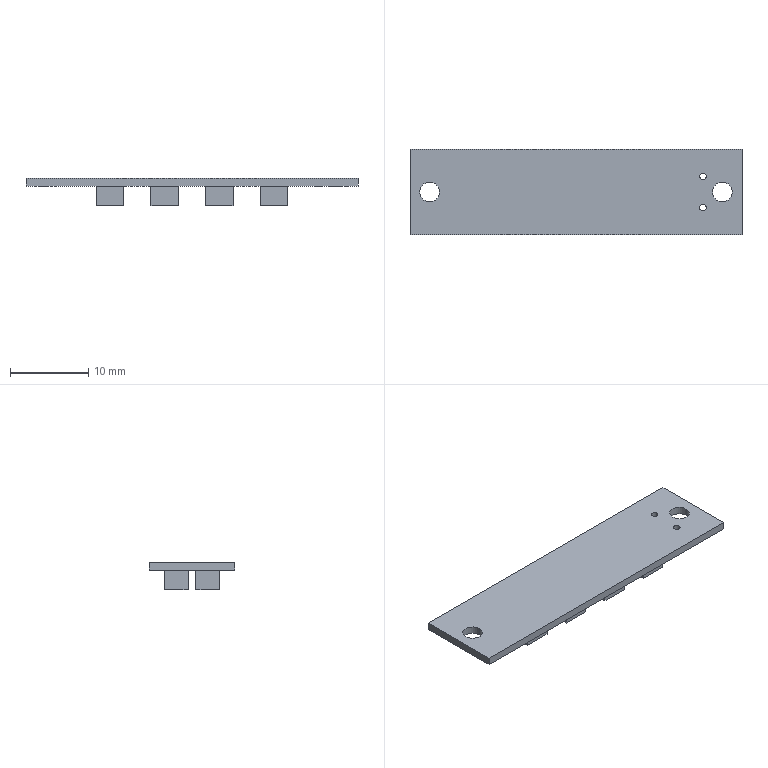Part | STEP file | LED lamp | 1 solid | 54 faces | box 42.5 x 11 x 3.5 mm | volume 662.951 mm3 | plane 46 | cylinder 8 | commonest cylinder face diameters 2.5 x4 0.838 x2 0.855 x2
STEP:
#1=CARTESIAN_POINT('',(27.178,-4.,3.5));
#2=VERTEX_POINT('',#1);
#3=CARTESIAN_POINT('',(26.322,-4.,3.5));
#4=VERTEX_POINT('',#3);
#5=CARTESIAN_POINT('',(26.75,-4.,3.5));
#6=DIRECTION('',(0.,0.,-1.));
#7=DIRECTION('',(-1.,0.,0.));
#8=AXIS2_PLACEMENT_3D('',#5,#6,#7);
#9=CIRCLE('',#8,0.4275);
#10=EDGE_CURVE('',#2,#4,#9,.T.);
#11=ORIENTED_EDGE('',*,*,#10,.F.);
#12=CARTESIAN_POINT('',(27.178,-4.,2.5));
#13=VERTEX_POINT('',#12);
#14=CARTESIAN_POINT('',(27.178,-4.,3.5));
#15=DIRECTION('',(0.,0.,-1.));
#16=VECTOR('',#15,1000.);
#17=LINE('',#14,#16);
#18=EDGE_CURVE('',#2,#13,#17,.T.);
#19=ORIENTED_EDGE('',*,*,#18,.T.);
#20=CARTESIAN_POINT('',(26.322,-4.,2.5));
#21=VERTEX_POINT('',#20);
#22=CARTESIAN_POINT('',(26.75,-4.,2.5));
#23=DIRECTION('',(0.,0.,-1.));
#24=DIRECTION('',(-1.,0.,0.));
#25=AXIS2_PLACEMENT_3D('',#22,#23,#24);
#26=CIRCLE('',#25,0.4275);
#27=EDGE_CURVE('',#13,#21,#26,.T.);
#28=ORIENTED_EDGE('',*,*,#27,.T.);
#29=CARTESIAN_POINT('',(26.322,-4.,3.5));
#30=DIRECTION('',(0.,0.,-1.));
#31=VECTOR('',#30,1000.);
#32=LINE('',#29,#31);
#33=EDGE_CURVE('',#4,#21,#32,.T.);
#34=ORIENTED_EDGE('',*,*,#33,.F.);
#35=EDGE_LOOP('',(#11,#19,#28,#34));
#36=FACE_OUTER_BOUND('',#35,.T.);
#37=CARTESIAN_POINT('',(26.75,-4.,3.5));
#38=DIRECTION('',(0.,0.,-1.));
#39=DIRECTION('',(-1.,0.,0.));
#40=AXIS2_PLACEMENT_3D('',#37,#38,#39);
#41=CYLINDRICAL_SURFACE('',#40,0.4275);
#42=ADVANCED_FACE('',(#36),#41,.F.);
#43=CARTESIAN_POINT('',(27.169,0.,3.5));
#44=VERTEX_POINT('',#43);
#45=CARTESIAN_POINT('',(26.331,0.,3.5));
#46=VERTEX_POINT('',#45);
#47=CARTESIAN_POINT('',(26.75,0.,3.5));
#48=DIRECTION('',(0.,0.,-1.));
#49=DIRECTION('',(-1.,0.,0.));
#50=AXIS2_PLACEMENT_3D('',#47,#48,#49);
#51=CIRCLE('',#50,0.4192);
#52=EDGE_CURVE('',#44,#46,#51,.T.);
#53=ORIENTED_EDGE('',*,*,#52,.F.);
#54=CARTESIAN_POINT('',(27.169,0.,2.5));
#55=VERTEX_POINT('',#54);
#56=CARTESIAN_POINT('',(27.169,0.,3.5));
#57=DIRECTION('',(0.,0.,-1.));
#58=VECTOR('',#57,1000.);
#59=LINE('',#56,#58);
#60=EDGE_CURVE('',#44,#55,#59,.T.);
#61=ORIENTED_EDGE('',*,*,#60,.T.);
#62=CARTESIAN_POINT('',(26.331,0.,2.5));
#63=VERTEX_POINT('',#62);
#64=CARTESIAN_POINT('',(26.75,0.,2.5));
#65=DIRECTION('',(0.,0.,-1.));
#66=DIRECTION('',(-1.,0.,0.));
#67=AXIS2_PLACEMENT_3D('',#64,#65,#66);
#68=CIRCLE('',#67,0.4192);
#69=EDGE_CURVE('',#55,#63,#68,.T.);
#70=ORIENTED_EDGE('',*,*,#69,.T.);
#71=CARTESIAN_POINT('',(26.331,0.,3.5));
#72=DIRECTION('',(0.,0.,-1.));
#73=VECTOR('',#72,1000.);
#74=LINE('',#71,#73);
#75=EDGE_CURVE('',#46,#63,#74,.T.);
#76=ORIENTED_EDGE('',*,*,#75,.F.);
#77=EDGE_LOOP('',(#53,#61,#70,#76));
#78=FACE_OUTER_BOUND('',#77,.T.);
#79=CARTESIAN_POINT('',(26.75,0.,3.5));
#80=DIRECTION('',(0.,0.,-1.));
#81=DIRECTION('',(-1.,0.,0.));
#82=AXIS2_PLACEMENT_3D('',#79,#80,#81);
#83=CYLINDRICAL_SURFACE('',#82,0.4192);
#84=ADVANCED_FACE('',(#78),#83,.F.);
#85=CARTESIAN_POINT('',(-7.,-2.,3.5));
#86=VERTEX_POINT('',#85);
#87=CARTESIAN_POINT('',(-9.5,-2.,3.5));
#88=VERTEX_POINT('',#87);
#89=CARTESIAN_POINT('',(-8.25,-2.,3.5));
#90=DIRECTION('',(0.,0.,-1.));
#91=DIRECTION('',(-1.,0.,0.));
#92=AXIS2_PLACEMENT_3D('',#89,#90,#91);
#93=CIRCLE('',#92,1.25);
#94=EDGE_CURVE('',#86,#88,#93,.T.);
#95=ORIENTED_EDGE('',*,*,#94,.F.);
#96=CARTESIAN_POINT('',(-7.,-2.,2.5));
#97=VERTEX_POINT('',#96);
#98=CARTESIAN_POINT('',(-7.,-2.,3.5));
#99=DIRECTION('',(0.,0.,-1.));
#100=VECTOR('',#99,1000.);
#101=LINE('',#98,#100);
#102=EDGE_CURVE('',#86,#97,#101,.T.);
#103=ORIENTED_EDGE('',*,*,#102,.T.);
#104=CARTESIAN_POINT('',(-9.5,-2.,2.5));
#105=VERTEX_POINT('',#104);
#106=CARTESIAN_POINT('',(-8.25,-2.,2.5));
#107=DIRECTION('',(0.,0.,-1.));
#108=DIRECTION('',(-1.,0.,0.));
#109=AXIS2_PLACEMENT_3D('',#106,#107,#108);
#110=CIRCLE('',#109,1.25);
#111=EDGE_CURVE('',#97,#105,#110,.T.);
#112=ORIENTED_EDGE('',*,*,#111,.T.);
#113=CARTESIAN_POINT('',(-9.5,-2.,3.5));
#114=DIRECTION('',(0.,0.,-1.));
#115=VECTOR('',#114,1000.);
#116=LINE('',#113,#115);
#117=EDGE_CURVE('',#88,#105,#116,.T.);
#118=ORIENTED_EDGE('',*,*,#117,.F.);
#119=EDGE_LOOP('',(#95,#103,#112,#118));
#120=FACE_OUTER_BOUND('',#119,.T.);
#121=CARTESIAN_POINT('',(-8.25,-2.,3.5));
#122=DIRECTION('',(0.,0.,-1.));
#123=DIRECTION('',(-1.,0.,0.));
#124=AXIS2_PLACEMENT_3D('',#121,#122,#123);
#125=CYLINDRICAL_SURFACE('',#124,1.25);
#126=ADVANCED_FACE('',(#120),#125,.F.);
#127=CARTESIAN_POINT('',(30.5,-2.,3.5));
#128=VERTEX_POINT('',#127);
#129=CARTESIAN_POINT('',(28.,-2.,3.5));
#130=VERTEX_POINT('',#129);
#131=CARTESIAN_POINT('',(29.25,-2.,3.5));
#132=DIRECTION('',(0.,0.,-1.));
#133=DIRECTION('',(-1.,0.,0.));
#134=AXIS2_PLACEMENT_3D('',#131,#132,#133);
#135=CIRCLE('',#134,1.25);
#136=EDGE_CURVE('',#128,#130,#135,.T.);
#137=ORIENTED_EDGE('',*,*,#136,.F.);
#138=CARTESIAN_POINT('',(30.5,-2.,2.5));
#139=VERTEX_POINT('',#138);
#140=CARTESIAN_POINT('',(30.5,-2.,3.5));
#141=DIRECTION('',(0.,0.,-1.));
#142=VECTOR('',#141,1000.);
#143=LINE('',#140,#142);
#144=EDGE_CURVE('',#128,#139,#143,.T.);
#145=ORIENTED_EDGE('',*,*,#144,.T.);
#146=CARTESIAN_POINT('',(28.,-2.,2.5));
#147=VERTEX_POINT('',#146);
#148=CARTESIAN_POINT('',(29.25,-2.,2.5));
#149=DIRECTION('',(0.,0.,-1.));
#150=DIRECTION('',(-1.,0.,0.));
#151=AXIS2_PLACEMENT_3D('',#148,#149,#150);
#152=CIRCLE('',#151,1.25);
#153=EDGE_CURVE('',#139,#147,#152,.T.);
#154=ORIENTED_EDGE('',*,*,#153,.T.);
#155=CARTESIAN_POINT('',(28.,-2.,3.5));
#156=DIRECTION('',(0.,0.,-1.));
#157=VECTOR('',#156,1000.);
#158=LINE('',#155,#157);
#159=EDGE_CURVE('',#130,#147,#158,.T.);
#160=ORIENTED_EDGE('',*,*,#159,.F.);
#161=EDGE_LOOP('',(#137,#145,#154,#160));
#162=FACE_OUTER_BOUND('',#161,.T.);
#163=CARTESIAN_POINT('',(29.25,-2.,3.5));
#164=DIRECTION('',(0.,0.,-1.));
#165=DIRECTION('',(-1.,0.,0.));
#166=AXIS2_PLACEMENT_3D('',#163,#164,#165);
#167=CYLINDRICAL_SURFACE('',#166,1.25);
#168=ADVANCED_FACE('',(#162),#167,.F.);
#169=CARTESIAN_POINT('',(26.75,-4.,2.5));
#170=DIRECTION('',(0.,0.,-1.));
#171=DIRECTION('',(-1.,0.,0.));
#172=AXIS2_PLACEMENT_3D('',#169,#170,#171);
#173=CIRCLE('',#172,0.4275);
#174=EDGE_CURVE('',#21,#13,#173,.T.);
#175=ORIENTED_EDGE('',*,*,#174,.F.);
#176=ORIENTED_EDGE('',*,*,#27,.F.);
#177=EDGE_LOOP('',(#175,#176));
#178=FACE_BOUND('',#177,.T.);
#179=CARTESIAN_POINT('',(26.75,0.,2.5));
#180=DIRECTION('',(0.,0.,-1.));
#181=DIRECTION('',(-1.,0.,0.));
#182=AXIS2_PLACEMENT_3D('',#179,#180,#181);
#183=CIRCLE('',#182,0.4192);
#184=EDGE_CURVE('',#63,#55,#183,.T.);
#185=ORIENTED_EDGE('',*,*,#184,.F.);
#186=ORIENTED_EDGE('',*,*,#69,.F.);
#187=EDGE_LOOP('',(#185,#186));
#188=FACE_BOUND('',#187,.T.);
#189=CARTESIAN_POINT('',(-8.25,-2.,2.5));
#190=DIRECTION('',(0.,0.,-1.));
#191=DIRECTION('',(-1.,0.,0.));
#192=AXIS2_PLACEMENT_3D('',#189,#190,#191);
#193=CIRCLE('',#192,1.25);
#194=EDGE_CURVE('',#105,#97,#193,.T.);
#195=ORIENTED_EDGE('',*,*,#194,.F.);
#196=ORIENTED_EDGE('',*,*,#111,.F.);
#197=EDGE_LOOP('',(#195,#196));
#198=FACE_BOUND('',#197,.T.);
#199=CARTESIAN_POINT('',(29.25,-2.,2.5));
#200=DIRECTION('',(0.,0.,-1.));
#201=DIRECTION('',(-1.,0.,0.));
#202=AXIS2_PLACEMENT_3D('',#199,#200,#201);
#203=CIRCLE('',#202,1.25);
#204=EDGE_CURVE('',#147,#139,#203,.T.);
#205=ORIENTED_EDGE('',*,*,#204,.F.);
#206=ORIENTED_EDGE('',*,*,#153,.F.);
#207=EDGE_LOOP('',(#205,#206));
#208=FACE_BOUND('',#207,.T.);
#209=CARTESIAN_POINT('',(12.25,-2.637,2.5));
#210=VERTEX_POINT('',#209);
#211=CARTESIAN_POINT('',(12.25,-5.5,2.5));
#212=VERTEX_POINT('',#211);
#213=CARTESIAN_POINT('',(12.25,-2.637,2.5));
#214=DIRECTION('',(0.,-1.,0.));
#215=VECTOR('',#214,1000.);
#216=LINE('',#213,#215);
#217=EDGE_CURVE('',#210,#212,#216,.T.);
#218=ORIENTED_EDGE('',*,*,#217,.T.);
#219=CARTESIAN_POINT('',(15.75,-5.5,2.5));
#220=VERTEX_POINT('',#219);
#221=CARTESIAN_POINT('',(12.25,-5.5,2.5));
#222=DIRECTION('',(1.,0.,0.));
#223=VECTOR('',#222,1000.);
#224=LINE('',#221,#223);
#225=EDGE_CURVE('',#212,#220,#224,.T.);
#226=ORIENTED_EDGE('',*,*,#225,.T.);
#227=CARTESIAN_POINT('',(15.75,-2.637,2.5));
#228=VERTEX_POINT('',#227);
#229=CARTESIAN_POINT('',(15.75,-2.637,2.5));
#230=DIRECTION('',(0.,1.,0.));
#231=VECTOR('',#230,1000.);
#232=LINE('',#229,#231);
#233=EDGE_CURVE('',#220,#228,#232,.T.);
#234=ORIENTED_EDGE('',*,*,#233,.T.);
#235=CARTESIAN_POINT('',(12.25,-2.637,2.5));
#236=DIRECTION('',(-1.,0.,0.));
#237=VECTOR('',#236,1000.);
#238=LINE('',#235,#237);
#239=EDGE_CURVE('',#228,#210,#238,.T.);
#240=ORIENTED_EDGE('',*,*,#239,.T.);
#241=EDGE_LOOP('',(#218,#226,#234,#240));
#242=FACE_BOUND('',#241,.T.);
#243=CARTESIAN_POINT('',(-1.75,-2.5,2.5));
#244=VERTEX_POINT('',#243);
#245=CARTESIAN_POINT('',(-1.75,-5.5,2.5));
#246=VERTEX_POINT('',#245);
#247=CARTESIAN_POINT('',(-1.75,-2.5,2.5));
#248=DIRECTION('',(0.,-1.,0.));
#249=VECTOR('',#248,1000.);
#250=LINE('',#247,#249);
#251=EDGE_CURVE('',#244,#246,#250,.T.);
#252=ORIENTED_EDGE('',*,*,#251,.T.);
#253=CARTESIAN_POINT('',(1.75,-5.5,2.5));
#254=VERTEX_POINT('',#253);
#255=CARTESIAN_POINT('',(-1.75,-5.5,2.5));
#256=DIRECTION('',(1.,0.,0.));
#257=VECTOR('',#256,1000.);
#258=LINE('',#255,#257);
#259=EDGE_CURVE('',#246,#254,#258,.T.);
#260=ORIENTED_EDGE('',*,*,#259,.T.);
#261=CARTESIAN_POINT('',(1.75,-2.5,2.5));
#262=VERTEX_POINT('',#261);
#263=CARTESIAN_POINT('',(1.75,-2.5,2.5));
#264=DIRECTION('',(0.,1.,0.));
#265=VECTOR('',#264,1000.);
#266=LINE('',#263,#265);
#267=EDGE_CURVE('',#254,#262,#266,.T.);
#268=ORIENTED_EDGE('',*,*,#267,.T.);
#269=CARTESIAN_POINT('',(-1.75,-2.5,2.5));
#270=DIRECTION('',(-1.,0.,0.));
#271=VECTOR('',#270,1000.);
#272=LINE('',#269,#271);
#273=EDGE_CURVE('',#262,#244,#272,.T.);
#274=ORIENTED_EDGE('',*,*,#273,.T.);
#275=EDGE_LOOP('',(#252,#260,#268,#274));
#276=FACE_BOUND('',#275,.T.);
#277=CARTESIAN_POINT('',(12.25,1.5,2.5));
#278=VERTEX_POINT('',#277);
#279=CARTESIAN_POINT('',(12.25,-1.5,2.5));
#280=VERTEX_POINT('',#279);
#281=CARTESIAN_POINT('',(12.25,1.5,2.5));
#282=DIRECTION('',(0.,-1.,0.));
#283=VECTOR('',#282,1000.);
#284=LINE('',#281,#283);
#285=EDGE_CURVE('',#278,#280,#284,.T.);
#286=ORIENTED_EDGE('',*,*,#285,.T.);
#287=CARTESIAN_POINT('',(15.75,-1.5,2.5));
#288=VERTEX_POINT('',#287);
#289=CARTESIAN_POINT('',(12.25,-1.5,2.5));
#290=DIRECTION('',(1.,0.,0.));
#291=VECTOR('',#290,1000.);
#292=LINE('',#289,#291);
#293=EDGE_CURVE('',#280,#288,#292,.T.);
#294=ORIENTED_EDGE('',*,*,#293,.T.);
#295=CARTESIAN_POINT('',(15.75,1.5,2.5));
#296=VERTEX_POINT('',#295);
#297=CARTESIAN_POINT('',(15.75,1.5,2.5));
#298=DIRECTION('',(0.,1.,0.));
#299=VECTOR('',#298,1000.);
#300=LINE('',#297,#299);
#301=EDGE_CURVE('',#288,#296,#300,.T.);
#302=ORIENTED_EDGE('',*,*,#301,.T.);
#303=CARTESIAN_POINT('',(12.25,1.5,2.5));
#304=DIRECTION('',(-1.,0.,0.));
#305=VECTOR('',#304,1000.);
#306=LINE('',#303,#305);
#307=EDGE_CURVE('',#296,#278,#306,.T.);
#308=ORIENTED_EDGE('',*,*,#307,.T.);
#309=EDGE_LOOP('',(#286,#294,#302,#308));
#310=FACE_BOUND('',#309,.T.);
#311=CARTESIAN_POINT('',(-1.75,-1.5,2.5));
#312=VERTEX_POINT('',#311);
#313=CARTESIAN_POINT('',(1.75,-1.5,2.5));
#314=VERTEX_POINT('',#313);
#315=CARTESIAN_POINT('',(-1.75,-1.5,2.5));
#316=DIRECTION('',(1.,0.,0.));
#317=VECTOR('',#316,1000.);
#318=LINE('',#315,#317);
#319=EDGE_CURVE('',#312,#314,#318,.T.);
#320=ORIENTED_EDGE('',*,*,#319,.T.);
#321=CARTESIAN_POINT('',(1.75,1.5,2.5));
#322=VERTEX_POINT('',#321);
#323=CARTESIAN_POINT('',(1.75,1.5,2.5));
#324=DIRECTION('',(0.,1.,0.));
#325=VECTOR('',#324,1000.);
#326=LINE('',#323,#325);
#327=EDGE_CURVE('',#314,#322,#326,.T.);
#328=ORIENTED_EDGE('',*,*,#327,.T.);
#329=CARTESIAN_POINT('',(-1.75,1.5,2.5));
#330=VERTEX_POINT('',#329);
#331=CARTESIAN_POINT('',(-1.75,1.5,2.5));
#332=DIRECTION('',(-1.,0.,0.));
#333=VECTOR('',#332,1000.);
#334=LINE('',#331,#333);
#335=EDGE_CURVE('',#322,#330,#334,.T.);
#336=ORIENTED_EDGE('',*,*,#335,.T.);
#337=CARTESIAN_POINT('',(-1.75,1.5,2.5));
#338=DIRECTION('',(0.,-1.,0.));
#339=VECTOR('',#338,1000.);
#340=LINE('',#337,#339);
#341=EDGE_CURVE('',#330,#312,#340,.T.);
#342=ORIENTED_EDGE('',*,*,#341,.T.);
#343=EDGE_LOOP('',(#320,#328,#336,#342));
#344=FACE_BOUND('',#343,.T.);
#345=CARTESIAN_POINT('',(-10.75,3.5,2.5));
#346=VERTEX_POINT('',#345);
#347=CARTESIAN_POINT('',(-10.75,-7.5,2.5));
#348=VERTEX_POINT('',#347);
#349=CARTESIAN_POINT('',(-10.75,3.5,2.5));
#350=DIRECTION('',(0.,-1.,0.));
#351=VECTOR('',#350,1000.);
#352=LINE('',#349,#351);
#353=EDGE_CURVE('',#346,#348,#352,.T.);
#354=ORIENTED_EDGE('',*,*,#353,.F.);
#355=CARTESIAN_POINT('',(31.75,3.5,2.5));
#356=VERTEX_POINT('',#355);
#357=CARTESIAN_POINT('',(-10.75,3.5,2.5));
#358=DIRECTION('',(-1.,0.,0.));
#359=VECTOR('',#358,1000.);
#360=LINE('',#357,#359);
#361=EDGE_CURVE('',#356,#346,#360,.T.);
#362=ORIENTED_EDGE('',*,*,#361,.F.);
#363=CARTESIAN_POINT('',(31.75,-7.5,2.5));
#364=VERTEX_POINT('',#363);
#365=CARTESIAN_POINT('',(31.75,3.5,2.5));
#366=DIRECTION('',(0.,1.,0.));
#367=VECTOR('',#366,1000.);
#368=LINE('',#365,#367);
#369=EDGE_CURVE('',#364,#356,#368,.T.);
#370=ORIENTED_EDGE('',*,*,#369,.F.);
#371=CARTESIAN_POINT('',(-10.75,-7.5,2.5));
#372=DIRECTION('',(1.,0.,0.));
#373=VECTOR('',#372,1000.);
#374=LINE('',#371,#373);
#375=EDGE_CURVE('',#348,#364,#374,.T.);
#376=ORIENTED_EDGE('',*,*,#375,.F.);
#377=EDGE_LOOP('',(#354,#362,#370,#376));
#378=FACE_OUTER_BOUND('',#377,.T.);
#379=CARTESIAN_POINT('',(5.25,1.5,2.5));
#380=VERTEX_POINT('',#379);
#381=CARTESIAN_POINT('',(5.25,-1.5,2.5));
#382=VERTEX_POINT('',#381);
#383=CARTESIAN_POINT('',(5.25,1.5,2.5));
#384=DIRECTION('',(0.,-1.,0.));
#385=VECTOR('',#384,1000.);
#386=LINE('',#383,#385);
#387=EDGE_CURVE('',#380,#382,#386,.T.);
#388=ORIENTED_EDGE('',*,*,#387,.T.);
#389=CARTESIAN_POINT('',(8.75,-1.5,2.5));
#390=VERTEX_POINT('',#389);
#391=CARTESIAN_POINT('',(5.25,-1.5,2.5));
#392=DIRECTION('',(1.,0.,0.));
#393=VECTOR('',#392,1000.);
#394=LINE('',#391,#393);
#395=EDGE_CURVE('',#382,#390,#394,.T.);
#396=ORIENTED_EDGE('',*,*,#395,.T.);
#397=CARTESIAN_POINT('',(8.75,1.5,2.5));
#398=VERTEX_POINT('',#397);
#399=CARTESIAN_POINT('',(8.75,1.5,2.5));
#400=DIRECTION('',(0.,1.,0.));
#401=VECTOR('',#400,1000.);
#402=LINE('',#399,#401);
#403=EDGE_CURVE('',#390,#398,#402,.T.);
#404=ORIENTED_EDGE('',*,*,#403,.T.);
#405=CARTESIAN_POINT('',(5.25,1.5,2.5));
#406=DIRECTION('',(-1.,0.,0.));
#407=VECTOR('',#406,1000.);
#408=LINE('',#405,#407);
#409=EDGE_CURVE('',#398,#380,#408,.T.);
#410=ORIENTED_EDGE('',*,*,#409,.T.);
#411=EDGE_LOOP('',(#388,#396,#404,#410));
#412=FACE_BOUND('',#411,.T.);
#413=CARTESIAN_POINT('',(19.25,1.5,2.5));
#414=VERTEX_POINT('',#413);
#415=CARTESIAN_POINT('',(19.25,-1.5,2.5));
#416=VERTEX_POINT('',#415);
#417=CARTESIAN_POINT('',(19.25,1.5,2.5));
#418=DIRECTION('',(0.,-1.,0.));
#419=VECTOR('',#418,1000.);
#420=LINE('',#417,#419);
#421=EDGE_CURVE('',#414,#416,#420,.T.);
#422=ORIENTED_EDGE('',*,*,#421,.T.);
#423=CARTESIAN_POINT('',(22.75,-1.5,2.5));
#424=VERTEX_POINT('',#423);
#425=CARTESIAN_POINT('',(19.25,-1.5,2.5));
#426=DIRECTION('',(1.,0.,0.));
#427=VECTOR('',#426,1000.);
#428=LINE('',#425,#427);
#429=EDGE_CURVE('',#416,#424,#428,.T.);
#430=ORIENTED_EDGE('',*,*,#429,.T.);
#431=CARTESIAN_POINT('',(22.75,1.5,2.5));
#432=VERTEX_POINT('',#431);
#433=CARTESIAN_POINT('',(22.75,1.5,2.5));
#434=DIRECTION('',(0.,1.,0.));
#435=VECTOR('',#434,1000.);
#436=LINE('',#433,#435);
#437=EDGE_CURVE('',#424,#432,#436,.T.);
#438=ORIENTED_EDGE('',*,*,#437,.T.);
#439=CARTESIAN_POINT('',(19.25,1.5,2.5));
#440=DIRECTION('',(-1.,0.,0.));
#441=VECTOR('',#440,1000.);
#442=LINE('',#439,#441);
#443=EDGE_CURVE('',#432,#414,#442,.T.);
#444=ORIENTED_EDGE('',*,*,#443,.T.);
#445=EDGE_LOOP('',(#422,#430,#438,#444));
#446=FACE_BOUND('',#445,.T.);
#447=CARTESIAN_POINT('',(5.25,-2.637,2.5));
#448=VERTEX_POINT('',#447);
#449=CARTESIAN_POINT('',(5.25,-5.5,2.5));
#450=VERTEX_POINT('',#449);
#451=CARTESIAN_POINT('',(5.25,-2.637,2.5));
#452=DIRECTION('',(0.,-1.,0.));
#453=VECTOR('',#452,1000.);
#454=LINE('',#451,#453);
#455=EDGE_CURVE('',#448,#450,#454,.T.);
#456=ORIENTED_EDGE('',*,*,#455,.T.);
#457=CARTESIAN_POINT('',(8.75,-5.5,2.5));
#458=VERTEX_POINT('',#457);
#459=CARTESIAN_POINT('',(5.25,-5.5,2.5));
#460=DIRECTION('',(1.,0.,0.));
#461=VECTOR('',#460,1000.);
#462=LINE('',#459,#461);
#463=EDGE_CURVE('',#450,#458,#462,.T.);
#464=ORIENTED_EDGE('',*,*,#463,.T.);
#465=CARTESIAN_POINT('',(8.75,-2.637,2.5));
#466=VERTEX_POINT('',#465);
#467=CARTESIAN_POINT('',(8.75,-2.637,2.5));
#468=DIRECTION('',(0.,1.,0.));
#469=VECTOR('',#468,1000.);
#470=LINE('',#467,#469);
#471=EDGE_CURVE('',#458,#466,#470,.T.);
#472=ORIENTED_EDGE('',*,*,#471,.T.);
#473=CARTESIAN_POINT('',(5.25,-2.637,2.5));
#474=DIRECTION('',(-1.,0.,0.));
#475=VECTOR('',#474,1000.);
#476=LINE('',#473,#475);
#477=EDGE_CURVE('',#466,#448,#476,.T.);
#478=ORIENTED_EDGE('',*,*,#477,.T.);
#479=EDGE_LOOP('',(#456,#464,#472,#478));
#480=FACE_BOUND('',#479,.T.);
#481=CARTESIAN_POINT('',(19.25,-2.637,2.5));
#482=VERTEX_POINT('',#481);
#483=CARTESIAN_POINT('',(19.25,-5.5,2.5));
#484=VERTEX_POINT('',#483);
#485=CARTESIAN_POINT('',(19.25,-2.637,2.5));
#486=DIRECTION('',(0.,-1.,0.));
#487=VECTOR('',#486,1000.);
#488=LINE('',#485,#487);
#489=EDGE_CURVE('',#482,#484,#488,.T.);
#490=ORIENTED_EDGE('',*,*,#489,.T.);
#491=CARTESIAN_POINT('',(22.75,-5.5,2.5));
#492=VERTEX_POINT('',#491);
#493=CARTESIAN_POINT('',(19.25,-5.5,2.5));
#494=DIRECTION('',(1.,0.,0.));
#495=VECTOR('',#494,1000.);
#496=LINE('',#493,#495);
#497=EDGE_CURVE('',#484,#492,#496,.T.);
#498=ORIENTED_EDGE('',*,*,#497,.T.);
#499=CARTESIAN_POINT('',(22.75,-2.637,2.5));
#500=VERTEX_POINT('',#499);
#501=CARTESIAN_POINT('',(22.75,-2.637,2.5));
#502=DIRECTION('',(0.,1.,0.));
#503=VECTOR('',#502,1000.);
#504=LINE('',#501,#503);
#505=EDGE_CURVE('',#492,#500,#504,.T.);
#506=ORIENTED_EDGE('',*,*,#505,.T.);
#507=CARTESIAN_POINT('',(19.25,-2.637,2.5));
#508=DIRECTION('',(-1.,0.,0.));
#509=VECTOR('',#508,1000.);
#510=LINE('',#507,#509);
#511=EDGE_CURVE('',#500,#482,#510,.T.);
#512=ORIENTED_EDGE('',*,*,#511,.T.);
#513=EDGE_LOOP('',(#490,#498,#506,#512));
#514=FACE_BOUND('',#513,.T.);
#515=CARTESIAN_POINT('',(-10.75,-7.5,2.5));
#516=DIRECTION('',(0.,0.,1.));
#517=DIRECTION('',(1.,0.,0.));
#518=AXIS2_PLACEMENT_3D('',#515,#516,#517);
#519=PLANE('',#518);
#520=ADVANCED_FACE('',(#178,#188,#198,#208,#242,#276,#310,#344,#378,#412,#446,#480,#514),#519,.F.);
#521=CARTESIAN_POINT('',(1.75,-1.5,0.));
#522=VERTEX_POINT('',#521);
#523=CARTESIAN_POINT('',(1.75,1.5,0.));
#524=VERTEX_POINT('',#523);
#525=CARTESIAN_POINT('',(1.75,1.5,0.));
#526=DIRECTION('',(0.,1.,0.));
#527=VECTOR('',#526,1000.);
#528=LINE('',#525,#527);
#529=EDGE_CURVE('',#522,#524,#528,.T.);
#530=ORIENTED_EDGE('',*,*,#529,.T.);
#531=CARTESIAN_POINT('',(1.75,1.5,2.5));
#532=DIRECTION('',(0.,0.,-1.));
#533=VECTOR('',#532,1000.);
#534=LINE('',#531,#533);
#535=EDGE_CURVE('',#322,#524,#534,.T.);
#536=ORIENTED_EDGE('',*,*,#535,.F.);
#537=ORIENTED_EDGE('',*,*,#327,.F.);
#538=CARTESIAN_POINT('',(1.75,-1.5,2.5));
#539=DIRECTION('',(0.,0.,-1.));
#540=VECTOR('',#539,1000.);
#541=LINE('',#538,#540);
#542=EDGE_CURVE('',#314,#522,#541,.T.);
#543=ORIENTED_EDGE('',*,*,#542,.T.);
#544=EDGE_LOOP('',(#530,#536,#537,#543));
#545=FACE_OUTER_BOUND('',#544,.T.);
#546=CARTESIAN_POINT('',(1.75,1.5,2.5));
#547=DIRECTION('',(-1.,0.,0.));
#548=DIRECTION('',(0.,-1.,0.));
#549=AXIS2_PLACEMENT_3D('',#546,#547,#548);
#550=PLANE('',#549);
#551=ADVANCED_FACE('',(#545),#550,.F.);
#552=CARTESIAN_POINT('',(-1.75,1.5,0.));
#553=VERTEX_POINT('',#552);
#554=CARTESIAN_POINT('',(-1.75,1.5,0.));
#555=DIRECTION('',(-1.,0.,0.));
#556=VECTOR('',#555,1000.);
#557=LINE('',#554,#556);
#558=EDGE_CURVE('',#524,#553,#557,.T.);
#559=ORIENTED_EDGE('',*,*,#558,.T.);
#560=CARTESIAN_POINT('',(-1.75,1.5,2.5));
#561=DIRECTION('',(0.,0.,-1.));
#562=VECTOR('',#561,1000.);
#563=LINE('',#560,#562);
#564=EDGE_CURVE('',#330,#553,#563,.T.);
#565=ORIENTED_EDGE('',*,*,#564,.F.);
#566=ORIENTED_EDGE('',*,*,#335,.F.);
#567=ORIENTED_EDGE('',*,*,#535,.T.);
#568=EDGE_LOOP('',(#559,#565,#566,#567));
#569=FACE_OUTER_BOUND('',#568,.T.);
#570=CARTESIAN_POINT('',(-1.75,1.5,2.5));
#571=DIRECTION('',(0.,-1.,0.));
#572=DIRECTION('',(0.,0.,-1.));
#573=AXIS2_PLACEMENT_3D('',#570,#571,#572);
#574=PLANE('',#573);
#575=ADVANCED_FACE('',(#569),#574,.F.);
#576=CARTESIAN_POINT('',(-1.75,-1.5,0.));
#577=VERTEX_POINT('',#576);
#578=CARTESIAN_POINT('',(-1.75,1.5,0.));
#579=DIRECTION('',(0.,-1.,0.));
#580=VECTOR('',#579,1000.);
#581=LINE('',#578,#580);
#582=EDGE_CURVE('',#553,#577,#581,.T.);
#583=ORIENTED_EDGE('',*,*,#582,.T.);
#584=CARTESIAN_POINT('',(-1.75,-1.5,2.5));
#585=DIRECTION('',(0.,0.,-1.));
#586=VECTOR('',#585,1000.);
#587=LINE('',#584,#586);
#588=EDGE_CURVE('',#312,#577,#587,.T.);
#589=ORIENTED_EDGE('',*,*,#588,.F.);
#590=ORIENTED_EDGE('',*,*,#341,.F.);
#591=ORIENTED_EDGE('',*,*,#564,.T.);
#592=EDGE_LOOP('',(#583,#589,#590,#591));
#593=FACE_OUTER_BOUND('',#592,.T.);
#594=CARTESIAN_POINT('',(-1.75,1.5,2.5));
#595=DIRECTION('',(1.,0.,0.));
#596=DIRECTION('',(0.,1.,0.));
#597=AXIS2_PLACEMENT_3D('',#594,#595,#596);
#598=PLANE('',#597);
#599=ADVANCED_FACE('',(#593),#598,.F.);
#600=CARTESIAN_POINT('',(-1.75,-1.5,0.));
#601=DIRECTION('',(1.,0.,0.));
#602=VECTOR('',#601,1000.);
#603=LINE('',#600,#602);
#604=EDGE_CURVE('',#577,#522,#603,.T.);
#605=ORIENTED_EDGE('',*,*,#604,.T.);
#606=ORIENTED_EDGE('',*,*,#542,.F.);
#607=ORIENTED_EDGE('',*,*,#319,.F.);
#608=ORIENTED_EDGE('',*,*,#588,.T.);
#609=EDGE_LOOP('',(#605,#606,#607,#608));
#610=FACE_OUTER_BOUND('',#609,.T.);
#611=CARTESIAN_POINT('',(-1.75,-1.5,2.5));
#612=DIRECTION('',(0.,1.,0.));
#613=DIRECTION('',(0.,0.,1.));
#614=AXIS2_PLACEMENT_3D('',#611,#612,#613);
#615=PLANE('',#614);
#616=ADVANCED_FACE('',(#610),#615,.F.);
#617=ORIENTED_EDGE('',*,*,#529,.F.);
#618=ORIENTED_EDGE('',*,*,#604,.F.);
#619=ORIENTED_EDGE('',*,*,#582,.F.);
#620=ORIENTED_EDGE('',*,*,#558,.F.);
#621=EDGE_LOOP('',(#617,#618,#619,#620));
#622=FACE_OUTER_BOUND('',#621,.T.);
#623=CARTESIAN_POINT('',(1.75,-1.5,0.));
#624=DIRECTION('',(0.,0.,1.));
#625=DIRECTION('',(1.,0.,0.));
#626=AXIS2_PLACEMENT_3D('',#623,#624,#625);
#627=PLANE('',#626);
#628=ADVANCED_FACE('',(#622),#627,.F.);
#629=ORIENTED_EDGE('',*,*,#353,.T.);
#630=CARTESIAN_POINT('',(-10.75,-7.5,3.5));
#631=VERTEX_POINT('',#630);
#632=CARTESIAN_POINT('',(-10.75,-7.5,3.5));
#633=DIRECTION('',(0.,0.,-1.));
#634=VECTOR('',#633,1000.);
#635=LINE('',#632,#634);
#636=EDGE_CURVE('',#631,#348,#635,.T.);
#637=ORIENTED_EDGE('',*,*,#636,.F.);
#638=CARTESIAN_POINT('',(-10.75,3.5,3.5));
#639=VERTEX_POINT('',#638);
#640=CARTESIAN_POINT('',(-10.75,3.5,3.5));
#641=DIRECTION('',(0.,-1.,0.));
#642=VECTOR('',#641,1000.);
#643=LINE('',#640,#642);
#644=EDGE_CURVE('',#639,#631,#643,.T.);
#645=ORIENTED_EDGE('',*,*,#644,.F.);
#646=CARTESIAN_POINT('',(-10.75,3.5,3.5));
#647=DIRECTION('',(0.,0.,-1.));
#648=VECTOR('',#647,1000.);
#649=LINE('',#646,#648);
#650=EDGE_CURVE('',#639,#346,#649,.T.);
#651=ORIENTED_EDGE('',*,*,#650,.T.);
#652=EDGE_LOOP('',(#629,#637,#645,#651));
#653=FACE_OUTER_BOUND('',#652,.T.);
#654=CARTESIAN_POINT('',(-10.75,3.5,3.5));
#655=DIRECTION('',(1.,0.,0.));
#656=DIRECTION('',(0.,1.,0.));
#657=AXIS2_PLACEMENT_3D('',#654,#655,#656);
#658=PLANE('',#657);
#659=ADVANCED_FACE('',(#653),#658,.F.);
#660=ORIENTED_EDGE('',*,*,#375,.T.);
#661=CARTESIAN_POINT('',(31.75,-7.5,3.5));
#662=VERTEX_POINT('',#661);
#663=CARTESIAN_POINT('',(31.75,-7.5,3.5));
#664=DIRECTION('',(0.,0.,-1.));
#665=VECTOR('',#664,1000.);
#666=LINE('',#663,#665);
#667=EDGE_CURVE('',#662,#364,#666,.T.);
#668=ORIENTED_EDGE('',*,*,#667,.F.);
#669=CARTESIAN_POINT('',(-10.75,-7.5,3.5));
#670=DIRECTION('',(1.,0.,0.));
#671=VECTOR('',#670,1000.);
#672=LINE('',#669,#671);
#673=EDGE_CURVE('',#631,#662,#672,.T.);
#674=ORIENTED_EDGE('',*,*,#673,.F.);
#675=ORIENTED_EDGE('',*,*,#636,.T.);
#676=EDGE_LOOP('',(#660,#668,#674,#675));
#677=FACE_OUTER_BOUND('',#676,.T.);
#678=CARTESIAN_POINT('',(-10.75,-7.5,3.5));
#679=DIRECTION('',(0.,1.,0.));
#680=DIRECTION('',(0.,0.,1.));
#681=AXIS2_PLACEMENT_3D('',#678,#679,#680);
#682=PLANE('',#681);
#683=ADVANCED_FACE('',(#677),#682,.F.);
#684=ORIENTED_EDGE('',*,*,#369,.T.);
#685=CARTESIAN_POINT('',(31.75,3.5,3.5));
#686=VERTEX_POINT('',#685);
#687=CARTESIAN_POINT('',(31.75,3.5,3.5));
#688=DIRECTION('',(0.,0.,-1.));
#689=VECTOR('',#688,1000.);
#690=LINE('',#687,#689);
#691=EDGE_CURVE('',#686,#356,#690,.T.);
#692=ORIENTED_EDGE('',*,*,#691,.F.);
#693=CARTESIAN_POINT('',(31.75,3.5,3.5));
#694=DIRECTION('',(0.,1.,0.));
#695=VECTOR('',#694,1000.);
#696=LINE('',#693,#695);
#697=EDGE_CURVE('',#662,#686,#696,.T.);
#698=ORIENTED_EDGE('',*,*,#697,.F.);
#699=ORIENTED_EDGE('',*,*,#667,.T.);
#700=EDGE_LOOP('',(#684,#692,#698,#699));
#701=FACE_OUTER_BOUND('',#700,.T.);
#702=CARTESIAN_POINT('',(31.75,3.5,3.5));
#703=DIRECTION('',(-1.,0.,0.));
#704=DIRECTION('',(0.,0.,1.));
#705=AXIS2_PLACEMENT_3D('',#702,#703,#704);
#706=PLANE('',#705);
#707=ADVANCED_FACE('',(#701),#706,.F.);
#708=ORIENTED_EDGE('',*,*,#361,.T.);
#709=ORIENTED_EDGE('',*,*,#650,.F.);
#710=CARTESIAN_POINT('',(-10.75,3.5,3.5));
#711=DIRECTION('',(-1.,0.,0.));
#712=VECTOR('',#711,1000.);
#713=LINE('',#710,#712);
#714=EDGE_CURVE('',#686,#639,#713,.T.);
#715=ORIENTED_EDGE('',*,*,#714,.F.);
#716=ORIENTED_EDGE('',*,*,#691,.T.);
#717=EDGE_LOOP('',(#708,#709,#715,#716));
#718=FACE_OUTER_BOUND('',#717,.T.);
#719=CARTESIAN_POINT('',(-10.75,3.5,3.5));
#720=DIRECTION('',(0.,-1.,0.));
#721=DIRECTION('',(0.,0.,-1.));
#722=AXIS2_PLACEMENT_3D('',#719,#720,#721);
#723=PLANE('',#722);
#724=ADVANCED_FACE('',(#718),#723,.F.);
#725=CARTESIAN_POINT('',(26.75,-4.,3.5));
#726=DIRECTION('',(0.,0.,-1.));
#727=DIRECTION('',(-1.,0.,0.));
#728=AXIS2_PLACEMENT_3D('',#725,#726,#727);
#729=CIRCLE('',#728,0.4275);
#730=EDGE_CURVE('',#4,#2,#729,.T.);
#731=ORIENTED_EDGE('',*,*,#730,.T.);
#732=ORIENTED_EDGE('',*,*,#10,.T.);
#733=EDGE_LOOP('',(#731,#732));
#734=FACE_BOUND('',#733,.T.);
#735=CARTESIAN_POINT('',(26.75,0.,3.5));
#736=DIRECTION('',(0.,0.,-1.));
#737=DIRECTION('',(-1.,0.,0.));
#738=AXIS2_PLACEMENT_3D('',#735,#736,#737);
#739=CIRCLE('',#738,0.4192);
#740=EDGE_CURVE('',#46,#44,#739,.T.);
#741=ORIENTED_EDGE('',*,*,#740,.T.);
#742=ORIENTED_EDGE('',*,*,#52,.T.);
#743=EDGE_LOOP('',(#741,#742));
#744=FACE_BOUND('',#743,.T.);
#745=CARTESIAN_POINT('',(-8.25,-2.,3.5));
#746=DIRECTION('',(0.,0.,-1.));
#747=DIRECTION('',(-1.,0.,0.));
#748=AXIS2_PLACEMENT_3D('',#745,#746,#747);
#749=CIRCLE('',#748,1.25);
#750=EDGE_CURVE('',#88,#86,#749,.T.);
#751=ORIENTED_EDGE('',*,*,#750,.T.);
#752=ORIENTED_EDGE('',*,*,#94,.T.);
#753=EDGE_LOOP('',(#751,#752));
#754=FACE_BOUND('',#753,.T.);
#755=CARTESIAN_POINT('',(29.25,-2.,3.5));
#756=DIRECTION('',(0.,0.,-1.));
#757=DIRECTION('',(-1.,0.,0.));
#758=AXIS2_PLACEMENT_3D('',#755,#756,#757);
#759=CIRCLE('',#758,1.25);
#760=EDGE_CURVE('',#130,#128,#759,.T.);
#761=ORIENTED_EDGE('',*,*,#760,.T.);
#762=ORIENTED_EDGE('',*,*,#136,.T.);
#763=EDGE_LOOP('',(#761,#762));
#764=FACE_BOUND('',#763,.T.);
#765=ORIENTED_EDGE('',*,*,#644,.T.);
#766=ORIENTED_EDGE('',*,*,#673,.T.);
#767=ORIENTED_EDGE('',*,*,#697,.T.);
#768=ORIENTED_EDGE('',*,*,#714,.T.);
#769=EDGE_LOOP('',(#765,#766,#767,#768));
#770=FACE_OUTER_BOUND('',#769,.T.);
#771=CARTESIAN_POINT('',(-10.75,-7.5,3.5));
#772=DIRECTION('',(0.,0.,1.));
#773=DIRECTION('',(1.,0.,0.));
#774=AXIS2_PLACEMENT_3D('',#771,#772,#773);
#775=PLANE('',#774);
#776=ADVANCED_FACE('',(#734,#744,#754,#764,#770),#775,.T.);
#777=CARTESIAN_POINT('',(5.25,1.5,0.));
#778=VERTEX_POINT('',#777);
#779=CARTESIAN_POINT('',(5.25,-1.5,0.));
#780=VERTEX_POINT('',#779);
#781=CARTESIAN_POINT('',(5.25,1.5,0.));
#782=DIRECTION('',(0.,-1.,0.));
#783=VECTOR('',#782,1000.);
#784=LINE('',#781,#783);
#785=EDGE_CURVE('',#778,#780,#784,.T.);
#786=ORIENTED_EDGE('',*,*,#785,.T.);
#787=CARTESIAN_POINT('',(5.25,-1.5,2.5));
#788=DIRECTION('',(0.,0.,-1.));
#789=VECTOR('',#788,1000.);
#790=LINE('',#787,#789);
#791=EDGE_CURVE('',#382,#780,#790,.T.);
#792=ORIENTED_EDGE('',*,*,#791,.F.);
#793=ORIENTED_EDGE('',*,*,#387,.F.);
#794=CARTESIAN_POINT('',(5.25,1.5,2.5));
#795=DIRECTION('',(0.,0.,-1.));
#796=VECTOR('',#795,1000.);
#797=LINE('',#794,#796);
#798=EDGE_CURVE('',#380,#778,#797,.T.);
#799=ORIENTED_EDGE('',*,*,#798,.T.);
#800=EDGE_LOOP('',(#786,#792,#793,#799));
#801=FACE_OUTER_BOUND('',#800,.T.);
#802=CARTESIAN_POINT('',(5.25,1.5,2.5));
#803=DIRECTION('',(1.,0.,0.));
#804=DIRECTION('',(0.,0.,-1.));
#805=AXIS2_PLACEMENT_3D('',#802,#803,#804);
#806=PLANE('',#805);
#807=ADVANCED_FACE('',(#801),#806,.F.);
#808=CARTESIAN_POINT('',(8.75,-1.5,0.));
#809=VERTEX_POINT('',#808);
#810=CARTESIAN_POINT('',(5.25,-1.5,0.));
#811=DIRECTION('',(1.,0.,0.));
#812=VECTOR('',#811,1000.);
#813=LINE('',#810,#812);
#814=EDGE_CURVE('',#780,#809,#813,.T.);
#815=ORIENTED_EDGE('',*,*,#814,.T.);
#816=CARTESIAN_POINT('',(8.75,-1.5,2.5));
#817=DIRECTION('',(0.,0.,-1.));
#818=VECTOR('',#817,1000.);
#819=LINE('',#816,#818);
#820=EDGE_CURVE('',#390,#809,#819,.T.);
#821=ORIENTED_EDGE('',*,*,#820,.F.);
#822=ORIENTED_EDGE('',*,*,#395,.F.);
#823=ORIENTED_EDGE('',*,*,#791,.T.);
#824=EDGE_LOOP('',(#815,#821,#822,#823));
#825=FACE_OUTER_BOUND('',#824,.T.);
#826=CARTESIAN_POINT('',(5.25,-1.5,2.5));
#827=DIRECTION('',(0.,1.,0.));
#828=DIRECTION('',(0.,0.,1.));
#829=AXIS2_PLACEMENT_3D('',#826,#827,#828);
#830=PLANE('',#829);
#831=ADVANCED_FACE('',(#825),#830,.F.);
#832=CARTESIAN_POINT('',(8.75,1.5,0.));
#833=VERTEX_POINT('',#832);
#834=CARTESIAN_POINT('',(8.75,1.5,0.));
#835=DIRECTION('',(0.,1.,0.));
#836=VECTOR('',#835,1000.);
#837=LINE('',#834,#836);
#838=EDGE_CURVE('',#809,#833,#837,.T.);
#839=ORIENTED_EDGE('',*,*,#838,.T.);
#840=CARTESIAN_POINT('',(8.75,1.5,2.5));
#841=DIRECTION('',(0.,0.,-1.));
#842=VECTOR('',#841,1000.);
#843=LINE('',#840,#842);
#844=EDGE_CURVE('',#398,#833,#843,.T.);
#845=ORIENTED_EDGE('',*,*,#844,.F.);
#846=ORIENTED_EDGE('',*,*,#403,.F.);
#847=ORIENTED_EDGE('',*,*,#820,.T.);
#848=EDGE_LOOP('',(#839,#845,#846,#847));
#849=FACE_OUTER_BOUND('',#848,.T.);
#850=CARTESIAN_POINT('',(8.75,1.5,2.5));
#851=DIRECTION('',(-1.,0.,0.));
#852=DIRECTION('',(0.,0.,1.));
#853=AXIS2_PLACEMENT_3D('',#850,#851,#852);
#854=PLANE('',#853);
#855=ADVANCED_FACE('',(#849),#854,.F.);
#856=CARTESIAN_POINT('',(5.25,1.5,0.));
#857=DIRECTION('',(-1.,0.,0.));
#858=VECTOR('',#857,1000.);
#859=LINE('',#856,#858);
#860=EDGE_CURVE('',#833,#778,#859,.T.);
#861=ORIENTED_EDGE('',*,*,#860,.T.);
#862=ORIENTED_EDGE('',*,*,#798,.F.);
#863=ORIENTED_EDGE('',*,*,#409,.F.);
#864=ORIENTED_EDGE('',*,*,#844,.T.);
#865=EDGE_LOOP('',(#861,#862,#863,#864));
#866=FACE_OUTER_BOUND('',#865,.T.);
#867=CARTESIAN_POINT('',(5.25,1.5,2.5));
#868=DIRECTION('',(0.,-1.,0.));
#869=DIRECTION('',(1.,0.,0.));
#870=AXIS2_PLACEMENT_3D('',#867,#868,#869);
#871=PLANE('',#870);
#872=ADVANCED_FACE('',(#866),#871,.F.);
#873=ORIENTED_EDGE('',*,*,#785,.F.);
#874=ORIENTED_EDGE('',*,*,#860,.F.);
#875=ORIENTED_EDGE('',*,*,#838,.F.);
#876=ORIENTED_EDGE('',*,*,#814,.F.);
#877=EDGE_LOOP('',(#873,#874,#875,#876));
#878=FACE_OUTER_BOUND('',#877,.T.);
#879=CARTESIAN_POINT('',(5.25,-1.5,0.));
#880=DIRECTION('',(0.,0.,1.));
#881=DIRECTION('',(1.,0.,0.));
#882=AXIS2_PLACEMENT_3D('',#879,#880,#881);
#883=PLANE('',#882);
#884=ADVANCED_FACE('',(#878),#883,.F.);
#885=CARTESIAN_POINT('',(12.25,1.5,0.));
#886=VERTEX_POINT('',#885);
#887=CARTESIAN_POINT('',(12.25,-1.5,0.));
#888=VERTEX_POINT('',#887);
#889=CARTESIAN_POINT('',(12.25,1.5,0.));
#890=DIRECTION('',(0.,-1.,0.));
#891=VECTOR('',#890,1000.);
#892=LINE('',#889,#891);
#893=EDGE_CURVE('',#886,#888,#892,.T.);
#894=ORIENTED_EDGE('',*,*,#893,.T.);
#895=CARTESIAN_POINT('',(12.25,-1.5,2.5));
#896=DIRECTION('',(0.,0.,-1.));
#897=VECTOR('',#896,1000.);
#898=LINE('',#895,#897);
#899=EDGE_CURVE('',#280,#888,#898,.T.);
#900=ORIENTED_EDGE('',*,*,#899,.F.);
#901=ORIENTED_EDGE('',*,*,#285,.F.);
#902=CARTESIAN_POINT('',(12.25,1.5,2.5));
#903=DIRECTION('',(0.,0.,-1.));
#904=VECTOR('',#903,1000.);
#905=LINE('',#902,#904);
#906=EDGE_CURVE('',#278,#886,#905,.T.);
#907=ORIENTED_EDGE('',*,*,#906,.T.);
#908=EDGE_LOOP('',(#894,#900,#901,#907));
#909=FACE_OUTER_BOUND('',#908,.T.);
#910=CARTESIAN_POINT('',(12.25,1.5,2.5));
#911=DIRECTION('',(1.,0.,0.));
#912=DIRECTION('',(0.,0.,-1.));
#913=AXIS2_PLACEMENT_3D('',#910,#911,#912);
#914=PLANE('',#913);
#915=ADVANCED_FACE('',(#909),#914,.F.);
#916=CARTESIAN_POINT('',(15.75,-1.5,0.));
#917=VERTEX_POINT('',#916);
#918=CARTESIAN_POINT('',(12.25,-1.5,0.));
#919=DIRECTION('',(1.,0.,0.));
#920=VECTOR('',#919,1000.);
#921=LINE('',#918,#920);
#922=EDGE_CURVE('',#888,#917,#921,.T.);
#923=ORIENTED_EDGE('',*,*,#922,.T.);
#924=CARTESIAN_POINT('',(15.75,-1.5,2.5));
#925=DIRECTION('',(0.,0.,-1.));
#926=VECTOR('',#925,1000.);
#927=LINE('',#924,#926);
#928=EDGE_CURVE('',#288,#917,#927,.T.);
#929=ORIENTED_EDGE('',*,*,#928,.F.);
#930=ORIENTED_EDGE('',*,*,#293,.F.);
#931=ORIENTED_EDGE('',*,*,#899,.T.);
#932=EDGE_LOOP('',(#923,#929,#930,#931));
#933=FACE_OUTER_BOUND('',#932,.T.);
#934=CARTESIAN_POINT('',(12.25,-1.5,2.5));
#935=DIRECTION('',(0.,1.,0.));
#936=DIRECTION('',(0.,0.,1.));
#937=AXIS2_PLACEMENT_3D('',#934,#935,#936);
#938=PLANE('',#937);
#939=ADVANCED_FACE('',(#933),#938,.F.);
#940=CARTESIAN_POINT('',(15.75,1.5,0.));
#941=VERTEX_POINT('',#940);
#942=CARTESIAN_POINT('',(15.75,1.5,0.));
#943=DIRECTION('',(0.,1.,0.));
#944=VECTOR('',#943,1000.);
#945=LINE('',#942,#944);
#946=EDGE_CURVE('',#917,#941,#945,.T.);
#947=ORIENTED_EDGE('',*,*,#946,.T.);
#948=CARTESIAN_POINT('',(15.75,1.5,2.5));
#949=DIRECTION('',(0.,0.,-1.));
#950=VECTOR('',#949,1000.);
#951=LINE('',#948,#950);
#952=EDGE_CURVE('',#296,#941,#951,.T.);
#953=ORIENTED_EDGE('',*,*,#952,.F.);
#954=ORIENTED_EDGE('',*,*,#301,.F.);
#955=ORIENTED_EDGE('',*,*,#928,.T.);
#956=EDGE_LOOP('',(#947,#953,#954,#955));
#957=FACE_OUTER_BOUND('',#956,.T.);
#958=CARTESIAN_POINT('',(15.75,1.5,2.5));
#959=DIRECTION('',(-1.,0.,0.));
#960=DIRECTION('',(0.,0.,1.));
#961=AXIS2_PLACEMENT_3D('',#958,#959,#960);
#962=PLANE('',#961);
#963=ADVANCED_FACE('',(#957),#962,.F.);
#964=CARTESIAN_POINT('',(12.25,1.5,0.));
#965=DIRECTION('',(-1.,0.,0.));
#966=VECTOR('',#965,1000.);
#967=LINE('',#964,#966);
#968=EDGE_CURVE('',#941,#886,#967,.T.);
#969=ORIENTED_EDGE('',*,*,#968,.T.);
#970=ORIENTED_EDGE('',*,*,#906,.F.);
#971=ORIENTED_EDGE('',*,*,#307,.F.);
#972=ORIENTED_EDGE('',*,*,#952,.T.);
#973=EDGE_LOOP('',(#969,#970,#971,#972));
#974=FACE_OUTER_BOUND('',#973,.T.);
#975=CARTESIAN_POINT('',(12.25,1.5,2.5));
#976=DIRECTION('',(0.,-1.,0.));
#977=DIRECTION('',(1.,0.,0.));
#978=AXIS2_PLACEMENT_3D('',#975,#976,#977);
#979=PLANE('',#978);
#980=ADVANCED_FACE('',(#974),#979,.F.);
#981=ORIENTED_EDGE('',*,*,#893,.F.);
#982=ORIENTED_EDGE('',*,*,#968,.F.);
#983=ORIENTED_EDGE('',*,*,#946,.F.);
#984=ORIENTED_EDGE('',*,*,#922,.F.);
#985=EDGE_LOOP('',(#981,#982,#983,#984));
#986=FACE_OUTER_BOUND('',#985,.T.);
#987=CARTESIAN_POINT('',(12.25,-1.5,0.));
#988=DIRECTION('',(0.,0.,1.));
#989=DIRECTION('',(1.,0.,0.));
#990=AXIS2_PLACEMENT_3D('',#987,#988,#989);
#991=PLANE('',#990);
#992=ADVANCED_FACE('',(#986),#991,.F.);
#993=CARTESIAN_POINT('',(19.25,1.5,0.));
#994=VERTEX_POINT('',#993);
#995=CARTESIAN_POINT('',(19.25,-1.5,0.));
#996=VERTEX_POINT('',#995);
#997=CARTESIAN_POINT('',(19.25,1.5,0.));
#998=DIRECTION('',(0.,-1.,0.));
#999=VECTOR('',#998,1000.);
#1000=LINE('',#997,#999);
#1001=EDGE_CURVE('',#994,#996,#1000,.T.);
#1002=ORIENTED_EDGE('',*,*,#1001,.T.);
#1003=CARTESIAN_POINT('',(19.25,-1.5,2.5));
#1004=DIRECTION('',(0.,0.,-1.));
#1005=VECTOR('',#1004,1000.);
#1006=LINE('',#1003,#1005);
#1007=EDGE_CURVE('',#416,#996,#1006,.T.);
#1008=ORIENTED_EDGE('',*,*,#1007,.F.);
#1009=ORIENTED_EDGE('',*,*,#421,.F.);
#1010=CARTESIAN_POINT('',(19.25,1.5,2.5));
#1011=DIRECTION('',(0.,0.,-1.));
#1012=VECTOR('',#1011,1000.);
#1013=LINE('',#1010,#1012);
#1014=EDGE_CURVE('',#414,#994,#1013,.T.);
#1015=ORIENTED_EDGE('',*,*,#1014,.T.);
#1016=EDGE_LOOP('',(#1002,#1008,#1009,#1015));
#1017=FACE_OUTER_BOUND('',#1016,.T.);
#1018=CARTESIAN_POINT('',(19.25,1.5,2.5));
#1019=DIRECTION('',(1.,0.,0.));
#1020=DIRECTION('',(0.,0.,-1.));
#1021=AXIS2_PLACEMENT_3D('',#1018,#1019,#1020);
#1022=PLANE('',#1021);
#1023=ADVANCED_FACE('',(#1017),#1022,.F.);
#1024=CARTESIAN_POINT('',(22.75,-1.5,0.));
#1025=VERTEX_POINT('',#1024);
#1026=CARTESIAN_POINT('',(19.25,-1.5,0.));
#1027=DIRECTION('',(1.,0.,0.));
#1028=VECTOR('',#1027,1000.);
#1029=LINE('',#1026,#1028);
#1030=EDGE_CURVE('',#996,#1025,#1029,.T.);
#1031=ORIENTED_EDGE('',*,*,#1030,.T.);
#1032=CARTESIAN_POINT('',(22.75,-1.5,2.5));
#1033=DIRECTION('',(0.,0.,-1.));
#1034=VECTOR('',#1033,1000.);
#1035=LINE('',#1032,#1034);
#1036=EDGE_CURVE('',#424,#1025,#1035,.T.);
#1037=ORIENTED_EDGE('',*,*,#1036,.F.);
#1038=ORIENTED_EDGE('',*,*,#429,.F.);
#1039=ORIENTED_EDGE('',*,*,#1007,.T.);
#1040=EDGE_LOOP('',(#1031,#1037,#1038,#1039));
#1041=FACE_OUTER_BOUND('',#1040,.T.);
#1042=CARTESIAN_POINT('',(19.25,-1.5,2.5));
#1043=DIRECTION('',(0.,1.,0.));
#1044=DIRECTION('',(-1.,0.,0.));
#1045=AXIS2_PLACEMENT_3D('',#1042,#1043,#1044);
#1046=PLANE('',#1045);
#1047=ADVANCED_FACE('',(#1041),#1046,.F.);
#1048=CARTESIAN_POINT('',(22.75,1.5,0.));
#1049=VERTEX_POINT('',#1048);
#1050=CARTESIAN_POINT('',(22.75,1.5,0.));
#1051=DIRECTION('',(0.,1.,0.));
#1052=VECTOR('',#1051,1000.);
#1053=LINE('',#1050,#1052);
#1054=EDGE_CURVE('',#1025,#1049,#1053,.T.);
#1055=ORIENTED_EDGE('',*,*,#1054,.T.);
#1056=CARTESIAN_POINT('',(22.75,1.5,2.5));
#1057=DIRECTION('',(0.,0.,-1.));
#1058=VECTOR('',#1057,1000.);
#1059=LINE('',#1056,#1058);
#1060=EDGE_CURVE('',#432,#1049,#1059,.T.);
#1061=ORIENTED_EDGE('',*,*,#1060,.F.);
#1062=ORIENTED_EDGE('',*,*,#437,.F.);
#1063=ORIENTED_EDGE('',*,*,#1036,.T.);
#1064=EDGE_LOOP('',(#1055,#1061,#1062,#1063));
#1065=FACE_OUTER_BOUND('',#1064,.T.);
#1066=CARTESIAN_POINT('',(22.75,1.5,2.5));
#1067=DIRECTION('',(-1.,0.,0.));
#1068=DIRECTION('',(0.,0.,1.));
#1069=AXIS2_PLACEMENT_3D('',#1066,#1067,#1068);
#1070=PLANE('',#1069);
#1071=ADVANCED_FACE('',(#1065),#1070,.F.);
#1072=CARTESIAN_POINT('',(19.25,1.5,0.));
#1073=DIRECTION('',(-1.,0.,0.));
#1074=VECTOR('',#1073,1000.);
#1075=LINE('',#1072,#1074);
#1076=EDGE_CURVE('',#1049,#994,#1075,.T.);
#1077=ORIENTED_EDGE('',*,*,#1076,.T.);
#1078=ORIENTED_EDGE('',*,*,#1014,.F.);
#1079=ORIENTED_EDGE('',*,*,#443,.F.);
#1080=ORIENTED_EDGE('',*,*,#1060,.T.);
#1081=EDGE_LOOP('',(#1077,#1078,#1079,#1080));
#1082=FACE_OUTER_BOUND('',#1081,.T.);
#1083=CARTESIAN_POINT('',(19.25,1.5,2.5));
#1084=DIRECTION('',(0.,-1.,0.));
#1085=DIRECTION('',(1.,0.,0.));
#1086=AXIS2_PLACEMENT_3D('',#1083,#1084,#1085);
#1087=PLANE('',#1086);
#1088=ADVANCED_FACE('',(#1082),#1087,.F.);
#1089=ORIENTED_EDGE('',*,*,#1001,.F.);
#1090=ORIENTED_EDGE('',*,*,#1076,.F.);
#1091=ORIENTED_EDGE('',*,*,#1054,.F.);
#1092=ORIENTED_EDGE('',*,*,#1030,.F.);
#1093=EDGE_LOOP('',(#1089,#1090,#1091,#1092));
#1094=FACE_OUTER_BOUND('',#1093,.T.);
#1095=CARTESIAN_POINT('',(19.25,-1.5,0.));
#1096=DIRECTION('',(0.,0.,1.));
#1097=DIRECTION('',(1.,0.,0.));
#1098=AXIS2_PLACEMENT_3D('',#1095,#1096,#1097);
#1099=PLANE('',#1098);
#1100=ADVANCED_FACE('',(#1094),#1099,.F.);
#1101=CARTESIAN_POINT('',(-1.75,-2.5,0.));
#1102=VERTEX_POINT('',#1101);
#1103=CARTESIAN_POINT('',(-1.75,-5.5,0.));
#1104=VERTEX_POINT('',#1103);
#1105=CARTESIAN_POINT('',(-1.75,-2.5,0.));
#1106=DIRECTION('',(0.,-1.,0.));
#1107=VECTOR('',#1106,1000.);
#1108=LINE('',#1105,#1107);
#1109=EDGE_CURVE('',#1102,#1104,#1108,.T.);
#1110=ORIENTED_EDGE('',*,*,#1109,.T.);
#1111=CARTESIAN_POINT('',(-1.75,-5.5,2.5));
#1112=DIRECTION('',(0.,0.,-1.));
#1113=VECTOR('',#1112,1000.);
#1114=LINE('',#1111,#1113);
#1115=EDGE_CURVE('',#246,#1104,#1114,.T.);
#1116=ORIENTED_EDGE('',*,*,#1115,.F.);
#1117=ORIENTED_EDGE('',*,*,#251,.F.);
#1118=CARTESIAN_POINT('',(-1.75,-2.5,2.5));
#1119=DIRECTION('',(0.,0.,-1.));
#1120=VECTOR('',#1119,1000.);
#1121=LINE('',#1118,#1120);
#1122=EDGE_CURVE('',#244,#1102,#1121,.T.);
#1123=ORIENTED_EDGE('',*,*,#1122,.T.);
#1124=EDGE_LOOP('',(#1110,#1116,#1117,#1123));
#1125=FACE_OUTER_BOUND('',#1124,.T.);
#1126=CARTESIAN_POINT('',(-1.75,-2.5,2.5));
#1127=DIRECTION('',(1.,0.,0.));
#1128=DIRECTION('',(0.,1.,0.));
#1129=AXIS2_PLACEMENT_3D('',#1126,#1127,#1128);
#1130=PLANE('',#1129);
#1131=ADVANCED_FACE('',(#1125),#1130,.F.);
#1132=CARTESIAN_POINT('',(1.75,-5.5,0.));
#1133=VERTEX_POINT('',#1132);
#1134=CARTESIAN_POINT('',(-1.75,-5.5,0.));
#1135=DIRECTION('',(1.,0.,0.));
#1136=VECTOR('',#1135,1000.);
#1137=LINE('',#1134,#1136);
#1138=EDGE_CURVE('',#1104,#1133,#1137,.T.);
#1139=ORIENTED_EDGE('',*,*,#1138,.T.);
#1140=CARTESIAN_POINT('',(1.75,-5.5,2.5));
#1141=DIRECTION('',(0.,0.,-1.));
#1142=VECTOR('',#1141,1000.);
#1143=LINE('',#1140,#1142);
#1144=EDGE_CURVE('',#254,#1133,#1143,.T.);
#1145=ORIENTED_EDGE('',*,*,#1144,.F.);
#1146=ORIENTED_EDGE('',*,*,#259,.F.);
#1147=ORIENTED_EDGE('',*,*,#1115,.T.);
#1148=EDGE_LOOP('',(#1139,#1145,#1146,#1147));
#1149=FACE_OUTER_BOUND('',#1148,.T.);
#1150=CARTESIAN_POINT('',(-1.75,-5.5,2.5));
#1151=DIRECTION('',(0.,1.,0.));
#1152=DIRECTION('',(0.,0.,1.));
#1153=AXIS2_PLACEMENT_3D('',#1150,#1151,#1152);
#1154=PLANE('',#1153);
#1155=ADVANCED_FACE('',(#1149),#1154,.F.);
#1156=CARTESIAN_POINT('',(1.75,-2.5,0.));
#1157=VERTEX_POINT('',#1156);
#1158=CARTESIAN_POINT('',(1.75,-2.5,0.));
#1159=DIRECTION('',(0.,1.,0.));
#1160=VECTOR('',#1159,1000.);
#1161=LINE('',#1158,#1160);
#1162=EDGE_CURVE('',#1133,#1157,#1161,.T.);
#1163=ORIENTED_EDGE('',*,*,#1162,.T.);
#1164=CARTESIAN_POINT('',(1.75,-2.5,2.5));
#1165=DIRECTION('',(0.,0.,-1.));
#1166=VECTOR('',#1165,1000.);
#1167=LINE('',#1164,#1166);
#1168=EDGE_CURVE('',#262,#1157,#1167,.T.);
#1169=ORIENTED_EDGE('',*,*,#1168,.F.);
#1170=ORIENTED_EDGE('',*,*,#267,.F.);
#1171=ORIENTED_EDGE('',*,*,#1144,.T.);
#1172=EDGE_LOOP('',(#1163,#1169,#1170,#1171));
#1173=FACE_OUTER_BOUND('',#1172,.T.);
#1174=CARTESIAN_POINT('',(1.75,-2.5,2.5));
#1175=DIRECTION('',(-1.,0.,0.));
#1176=DIRECTION('',(0.,-1.,0.));
#1177=AXIS2_PLACEMENT_3D('',#1174,#1175,#1176);
#1178=PLANE('',#1177);
#1179=ADVANCED_FACE('',(#1173),#1178,.F.);
#1180=CARTESIAN_POINT('',(-1.75,-2.5,0.));
#1181=DIRECTION('',(-1.,0.,0.));
#1182=VECTOR('',#1181,1000.);
#1183=LINE('',#1180,#1182);
#1184=EDGE_CURVE('',#1157,#1102,#1183,.T.);
#1185=ORIENTED_EDGE('',*,*,#1184,.T.);
#1186=ORIENTED_EDGE('',*,*,#1122,.F.);
#1187=ORIENTED_EDGE('',*,*,#273,.F.);
#1188=ORIENTED_EDGE('',*,*,#1168,.T.);
#1189=EDGE_LOOP('',(#1185,#1186,#1187,#1188));
#1190=FACE_OUTER_BOUND('',#1189,.T.);
#1191=CARTESIAN_POINT('',(-1.75,-2.5,2.5));
#1192=DIRECTION('',(0.,-1.,0.));
#1193=DIRECTION('',(0.,0.,-1.));
#1194=AXIS2_PLACEMENT_3D('',#1191,#1192,#1193);
#1195=PLANE('',#1194);
#1196=ADVANCED_FACE('',(#1190),#1195,.F.);
#1197=ORIENTED_EDGE('',*,*,#1109,.F.);
#1198=ORIENTED_EDGE('',*,*,#1184,.F.);
#1199=ORIENTED_EDGE('',*,*,#1162,.F.);
#1200=ORIENTED_EDGE('',*,*,#1138,.F.);
#1201=EDGE_LOOP('',(#1197,#1198,#1199,#1200));
#1202=FACE_OUTER_BOUND('',#1201,.T.);
#1203=CARTESIAN_POINT('',(-1.75,-5.5,0.));
#1204=DIRECTION('',(0.,0.,1.));
#1205=DIRECTION('',(1.,0.,0.));
#1206=AXIS2_PLACEMENT_3D('',#1203,#1204,#1205);
#1207=PLANE('',#1206);
#1208=ADVANCED_FACE('',(#1202),#1207,.F.);
#1209=CARTESIAN_POINT('',(5.25,-2.637,0.));
#1210=VERTEX_POINT('',#1209);
#1211=CARTESIAN_POINT('',(5.25,-5.5,0.));
#1212=VERTEX_POINT('',#1211);
#1213=CARTESIAN_POINT('',(5.25,-2.637,0.));
#1214=DIRECTION('',(0.,-1.,0.));
#1215=VECTOR('',#1214,1000.);
#1216=LINE('',#1213,#1215);
#1217=EDGE_CURVE('',#1210,#1212,#1216,.T.);
#1218=ORIENTED_EDGE('',*,*,#1217,.T.);
#1219=CARTESIAN_POINT('',(5.25,-5.5,2.5));
#1220=DIRECTION('',(0.,0.,-1.));
#1221=VECTOR('',#1220,1000.);
#1222=LINE('',#1219,#1221);
#1223=EDGE_CURVE('',#450,#1212,#1222,.T.);
#1224=ORIENTED_EDGE('',*,*,#1223,.F.);
#1225=ORIENTED_EDGE('',*,*,#455,.F.);
#1226=CARTESIAN_POINT('',(5.25,-2.637,2.5));
#1227=DIRECTION('',(0.,0.,-1.));
#1228=VECTOR('',#1227,1000.);
#1229=LINE('',#1226,#1228);
#1230=EDGE_CURVE('',#448,#1210,#1229,.T.);
#1231=ORIENTED_EDGE('',*,*,#1230,.T.);
#1232=EDGE_LOOP('',(#1218,#1224,#1225,#1231));
#1233=FACE_OUTER_BOUND('',#1232,.T.);
#1234=CARTESIAN_POINT('',(5.25,-2.637,2.5));
#1235=DIRECTION('',(1.,0.,0.));
#1236=DIRECTION('',(0.,1.,0.));
#1237=AXIS2_PLACEMENT_3D('',#1234,#1235,#1236);
#1238=PLANE('',#1237);
#1239=ADVANCED_FACE('',(#1233),#1238,.F.);
#1240=CARTESIAN_POINT('',(8.75,-5.5,0.));
#1241=VERTEX_POINT('',#1240);
#1242=CARTESIAN_POINT('',(5.25,-5.5,0.));
#1243=DIRECTION('',(1.,0.,0.));
#1244=VECTOR('',#1243,1000.);
#1245=LINE('',#1242,#1244);
#1246=EDGE_CURVE('',#1212,#1241,#1245,.T.);
#1247=ORIENTED_EDGE('',*,*,#1246,.T.);
#1248=CARTESIAN_POINT('',(8.75,-5.5,2.5));
#1249=DIRECTION('',(0.,0.,-1.));
#1250=VECTOR('',#1249,1000.);
#1251=LINE('',#1248,#1250);
#1252=EDGE_CURVE('',#458,#1241,#1251,.T.);
#1253=ORIENTED_EDGE('',*,*,#1252,.F.);
#1254=ORIENTED_EDGE('',*,*,#463,.F.);
#1255=ORIENTED_EDGE('',*,*,#1223,.T.);
#1256=EDGE_LOOP('',(#1247,#1253,#1254,#1255));
#1257=FACE_OUTER_BOUND('',#1256,.T.);
#1258=CARTESIAN_POINT('',(5.25,-5.5,2.5));
#1259=DIRECTION('',(0.,1.,0.));
#1260=DIRECTION('',(0.,0.,1.));
#1261=AXIS2_PLACEMENT_3D('',#1258,#1259,#1260);
#1262=PLANE('',#1261);
#1263=ADVANCED_FACE('',(#1257),#1262,.F.);
#1264=CARTESIAN_POINT('',(8.75,-2.637,0.));
#1265=VERTEX_POINT('',#1264);
#1266=CARTESIAN_POINT('',(8.75,-2.637,0.));
#1267=DIRECTION('',(0.,1.,0.));
#1268=VECTOR('',#1267,1000.);
#1269=LINE('',#1266,#1268);
#1270=EDGE_CURVE('',#1241,#1265,#1269,.T.);
#1271=ORIENTED_EDGE('',*,*,#1270,.T.);
#1272=CARTESIAN_POINT('',(8.75,-2.637,2.5));
#1273=DIRECTION('',(0.,0.,-1.));
#1274=VECTOR('',#1273,1000.);
#1275=LINE('',#1272,#1274);
#1276=EDGE_CURVE('',#466,#1265,#1275,.T.);
#1277=ORIENTED_EDGE('',*,*,#1276,.F.);
#1278=ORIENTED_EDGE('',*,*,#471,.F.);
#1279=ORIENTED_EDGE('',*,*,#1252,.T.);
#1280=EDGE_LOOP('',(#1271,#1277,#1278,#1279));
#1281=FACE_OUTER_BOUND('',#1280,.T.);
#1282=CARTESIAN_POINT('',(8.75,-2.637,2.5));
#1283=DIRECTION('',(-1.,0.,0.));
#1284=DIRECTION('',(0.,0.,1.));
#1285=AXIS2_PLACEMENT_3D('',#1282,#1283,#1284);
#1286=PLANE('',#1285);
#1287=ADVANCED_FACE('',(#1281),#1286,.F.);
#1288=CARTESIAN_POINT('',(5.25,-2.637,0.));
#1289=DIRECTION('',(-1.,0.,0.));
#1290=VECTOR('',#1289,1000.);
#1291=LINE('',#1288,#1290);
#1292=EDGE_CURVE('',#1265,#1210,#1291,.T.);
#1293=ORIENTED_EDGE('',*,*,#1292,.T.);
#1294=ORIENTED_EDGE('',*,*,#1230,.F.);
#1295=ORIENTED_EDGE('',*,*,#477,.F.);
#1296=ORIENTED_EDGE('',*,*,#1276,.T.);
#1297=EDGE_LOOP('',(#1293,#1294,#1295,#1296));
#1298=FACE_OUTER_BOUND('',#1297,.T.);
#1299=CARTESIAN_POINT('',(5.25,-2.637,2.5));
#1300=DIRECTION('',(0.,-1.,0.));
#1301=DIRECTION('',(0.,0.,-1.));
#1302=AXIS2_PLACEMENT_3D('',#1299,#1300,#1301);
#1303=PLANE('',#1302);
#1304=ADVANCED_FACE('',(#1298),#1303,.F.);
#1305=ORIENTED_EDGE('',*,*,#1217,.F.);
#1306=ORIENTED_EDGE('',*,*,#1292,.F.);
#1307=ORIENTED_EDGE('',*,*,#1270,.F.);
#1308=ORIENTED_EDGE('',*,*,#1246,.F.);
#1309=EDGE_LOOP('',(#1305,#1306,#1307,#1308));
#1310=FACE_OUTER_BOUND('',#1309,.T.);
#1311=CARTESIAN_POINT('',(5.25,-5.5,0.));
#1312=DIRECTION('',(0.,0.,1.));
#1313=DIRECTION('',(1.,0.,0.));
#1314=AXIS2_PLACEMENT_3D('',#1311,#1312,#1313);
#1315=PLANE('',#1314);
#1316=ADVANCED_FACE('',(#1310),#1315,.F.);
#1317=CARTESIAN_POINT('',(12.25,-2.637,0.));
#1318=VERTEX_POINT('',#1317);
#1319=CARTESIAN_POINT('',(12.25,-5.5,0.));
#1320=VERTEX_POINT('',#1319);
#1321=CARTESIAN_POINT('',(12.25,-2.637,0.));
#1322=DIRECTION('',(0.,-1.,0.));
#1323=VECTOR('',#1322,1000.);
#1324=LINE('',#1321,#1323);
#1325=EDGE_CURVE('',#1318,#1320,#1324,.T.);
#1326=ORIENTED_EDGE('',*,*,#1325,.T.);
#1327=CARTESIAN_POINT('',(12.25,-5.5,2.5));
#1328=DIRECTION('',(0.,0.,-1.));
#1329=VECTOR('',#1328,1000.);
#1330=LINE('',#1327,#1329);
#1331=EDGE_CURVE('',#212,#1320,#1330,.T.);
#1332=ORIENTED_EDGE('',*,*,#1331,.F.);
#1333=ORIENTED_EDGE('',*,*,#217,.F.);
#1334=CARTESIAN_POINT('',(12.25,-2.637,2.5));
#1335=DIRECTION('',(0.,0.,-1.));
#1336=VECTOR('',#1335,1000.);
#1337=LINE('',#1334,#1336);
#1338=EDGE_CURVE('',#210,#1318,#1337,.T.);
#1339=ORIENTED_EDGE('',*,*,#1338,.T.);
#1340=EDGE_LOOP('',(#1326,#1332,#1333,#1339));
#1341=FACE_OUTER_BOUND('',#1340,.T.);
#1342=CARTESIAN_POINT('',(12.25,-2.637,2.5));
#1343=DIRECTION('',(1.,0.,0.));
#1344=DIRECTION('',(0.,1.,0.));
#1345=AXIS2_PLACEMENT_3D('',#1342,#1343,#1344);
#1346=PLANE('',#1345);
#1347=ADVANCED_FACE('',(#1341),#1346,.F.);
#1348=CARTESIAN_POINT('',(15.75,-5.5,0.));
#1349=VERTEX_POINT('',#1348);
#1350=CARTESIAN_POINT('',(12.25,-5.5,0.));
#1351=DIRECTION('',(1.,0.,0.));
#1352=VECTOR('',#1351,1000.);
#1353=LINE('',#1350,#1352);
#1354=EDGE_CURVE('',#1320,#1349,#1353,.T.);
#1355=ORIENTED_EDGE('',*,*,#1354,.T.);
#1356=CARTESIAN_POINT('',(15.75,-5.5,2.5));
#1357=DIRECTION('',(0.,0.,-1.));
#1358=VECTOR('',#1357,1000.);
#1359=LINE('',#1356,#1358);
#1360=EDGE_CURVE('',#220,#1349,#1359,.T.);
#1361=ORIENTED_EDGE('',*,*,#1360,.F.);
#1362=ORIENTED_EDGE('',*,*,#225,.F.);
#1363=ORIENTED_EDGE('',*,*,#1331,.T.);
#1364=EDGE_LOOP('',(#1355,#1361,#1362,#1363));
#1365=FACE_OUTER_BOUND('',#1364,.T.);
#1366=CARTESIAN_POINT('',(12.25,-5.5,2.5));
#1367=DIRECTION('',(0.,1.,0.));
#1368=DIRECTION('',(0.,0.,1.));
#1369=AXIS2_PLACEMENT_3D('',#1366,#1367,#1368);
#1370=PLANE('',#1369);
#1371=ADVANCED_FACE('',(#1365),#1370,.F.);
#1372=CARTESIAN_POINT('',(15.75,-2.637,0.));
#1373=VERTEX_POINT('',#1372);
#1374=CARTESIAN_POINT('',(15.75,-2.637,0.));
#1375=DIRECTION('',(0.,1.,0.));
#1376=VECTOR('',#1375,1000.);
#1377=LINE('',#1374,#1376);
#1378=EDGE_CURVE('',#1349,#1373,#1377,.T.);
#1379=ORIENTED_EDGE('',*,*,#1378,.T.);
#1380=CARTESIAN_POINT('',(15.75,-2.637,2.5));
#1381=DIRECTION('',(0.,0.,-1.));
#1382=VECTOR('',#1381,1000.);
#1383=LINE('',#1380,#1382);
#1384=EDGE_CURVE('',#228,#1373,#1383,.T.);
#1385=ORIENTED_EDGE('',*,*,#1384,.F.);
#1386=ORIENTED_EDGE('',*,*,#233,.F.);
#1387=ORIENTED_EDGE('',*,*,#1360,.T.);
#1388=EDGE_LOOP('',(#1379,#1385,#1386,#1387));
#1389=FACE_OUTER_BOUND('',#1388,.T.);
#1390=CARTESIAN_POINT('',(15.75,-2.637,2.5));
#1391=DIRECTION('',(-1.,0.,0.));
#1392=DIRECTION('',(0.,0.,1.));
#1393=AXIS2_PLACEMENT_3D('',#1390,#1391,#1392);
#1394=PLANE('',#1393);
#1395=ADVANCED_FACE('',(#1389),#1394,.F.);
#1396=CARTESIAN_POINT('',(12.25,-2.637,0.));
#1397=DIRECTION('',(-1.,0.,0.));
#1398=VECTOR('',#1397,1000.);
#1399=LINE('',#1396,#1398);
#1400=EDGE_CURVE('',#1373,#1318,#1399,.T.);
#1401=ORIENTED_EDGE('',*,*,#1400,.T.);
#1402=ORIENTED_EDGE('',*,*,#1338,.F.);
#1403=ORIENTED_EDGE('',*,*,#239,.F.);
#1404=ORIENTED_EDGE('',*,*,#1384,.T.);
#1405=EDGE_LOOP('',(#1401,#1402,#1403,#1404));
#1406=FACE_OUTER_BOUND('',#1405,.T.);
#1407=CARTESIAN_POINT('',(12.25,-2.637,2.5));
#1408=DIRECTION('',(0.,-1.,0.));
#1409=DIRECTION('',(1.,0.,0.));
#1410=AXIS2_PLACEMENT_3D('',#1407,#1408,#1409);
#1411=PLANE('',#1410);
#1412=ADVANCED_FACE('',(#1406),#1411,.F.);
#1413=ORIENTED_EDGE('',*,*,#1325,.F.);
#1414=ORIENTED_EDGE('',*,*,#1400,.F.);
#1415=ORIENTED_EDGE('',*,*,#1378,.F.);
#1416=ORIENTED_EDGE('',*,*,#1354,.F.);
#1417=EDGE_LOOP('',(#1413,#1414,#1415,#1416));
#1418=FACE_OUTER_BOUND('',#1417,.T.);
#1419=CARTESIAN_POINT('',(12.25,-5.5,0.));
#1420=DIRECTION('',(0.,0.,1.));
#1421=DIRECTION('',(1.,0.,0.));
#1422=AXIS2_PLACEMENT_3D('',#1419,#1420,#1421);
#1423=PLANE('',#1422);
#1424=ADVANCED_FACE('',(#1418),#1423,.F.);
#1425=CARTESIAN_POINT('',(19.25,-2.637,0.));
#1426=VERTEX_POINT('',#1425);
#1427=CARTESIAN_POINT('',(19.25,-5.5,0.));
#1428=VERTEX_POINT('',#1427);
#1429=CARTESIAN_POINT('',(19.25,-2.637,0.));
#1430=DIRECTION('',(0.,-1.,0.));
#1431=VECTOR('',#1430,1000.);
#1432=LINE('',#1429,#1431);
#1433=EDGE_CURVE('',#1426,#1428,#1432,.T.);
#1434=ORIENTED_EDGE('',*,*,#1433,.T.);
#1435=CARTESIAN_POINT('',(19.25,-5.5,2.5));
#1436=DIRECTION('',(0.,0.,-1.));
#1437=VECTOR('',#1436,1000.);
#1438=LINE('',#1435,#1437);
#1439=EDGE_CURVE('',#484,#1428,#1438,.T.);
#1440=ORIENTED_EDGE('',*,*,#1439,.F.);
#1441=ORIENTED_EDGE('',*,*,#489,.F.);
#1442=CARTESIAN_POINT('',(19.25,-2.637,2.5));
#1443=DIRECTION('',(0.,0.,-1.));
#1444=VECTOR('',#1443,1000.);
#1445=LINE('',#1442,#1444);
#1446=EDGE_CURVE('',#482,#1426,#1445,.T.);
#1447=ORIENTED_EDGE('',*,*,#1446,.T.);
#1448=EDGE_LOOP('',(#1434,#1440,#1441,#1447));
#1449=FACE_OUTER_BOUND('',#1448,.T.);
#1450=CARTESIAN_POINT('',(19.25,-2.637,2.5));
#1451=DIRECTION('',(1.,0.,0.));
#1452=DIRECTION('',(0.,0.,-1.));
#1453=AXIS2_PLACEMENT_3D('',#1450,#1451,#1452);
#1454=PLANE('',#1453);
#1455=ADVANCED_FACE('',(#1449),#1454,.F.);
#1456=CARTESIAN_POINT('',(22.75,-5.5,0.));
#1457=VERTEX_POINT('',#1456);
#1458=CARTESIAN_POINT('',(19.25,-5.5,0.));
#1459=DIRECTION('',(1.,0.,0.));
#1460=VECTOR('',#1459,1000.);
#1461=LINE('',#1458,#1460);
#1462=EDGE_CURVE('',#1428,#1457,#1461,.T.);
#1463=ORIENTED_EDGE('',*,*,#1462,.T.);
#1464=CARTESIAN_POINT('',(22.75,-5.5,2.5));
#1465=DIRECTION('',(0.,0.,-1.));
#1466=VECTOR('',#1465,1000.);
#1467=LINE('',#1464,#1466);
#1468=EDGE_CURVE('',#492,#1457,#1467,.T.);
#1469=ORIENTED_EDGE('',*,*,#1468,.F.);
#1470=ORIENTED_EDGE('',*,*,#497,.F.);
#1471=ORIENTED_EDGE('',*,*,#1439,.T.);
#1472=EDGE_LOOP('',(#1463,#1469,#1470,#1471));
#1473=FACE_OUTER_BOUND('',#1472,.T.);
#1474=CARTESIAN_POINT('',(19.25,-5.5,2.5));
#1475=DIRECTION('',(0.,1.,0.));
#1476=DIRECTION('',(0.,0.,1.));
#1477=AXIS2_PLACEMENT_3D('',#1474,#1475,#1476);
#1478=PLANE('',#1477);
#1479=ADVANCED_FACE('',(#1473),#1478,.F.);
#1480=CARTESIAN_POINT('',(22.75,-2.637,0.));
#1481=VERTEX_POINT('',#1480);
#1482=CARTESIAN_POINT('',(22.75,-2.637,0.));
#1483=DIRECTION('',(0.,1.,0.));
#1484=VECTOR('',#1483,1000.);
#1485=LINE('',#1482,#1484);
#1486=EDGE_CURVE('',#1457,#1481,#1485,.T.);
#1487=ORIENTED_EDGE('',*,*,#1486,.T.);
#1488=CARTESIAN_POINT('',(22.75,-2.637,2.5));
#1489=DIRECTION('',(0.,0.,-1.));
#1490=VECTOR('',#1489,1000.);
#1491=LINE('',#1488,#1490);
#1492=EDGE_CURVE('',#500,#1481,#1491,.T.);
#1493=ORIENTED_EDGE('',*,*,#1492,.F.);
#1494=ORIENTED_EDGE('',*,*,#505,.F.);
#1495=ORIENTED_EDGE('',*,*,#1468,.T.);
#1496=EDGE_LOOP('',(#1487,#1493,#1494,#1495));
#1497=FACE_OUTER_BOUND('',#1496,.T.);
#1498=CARTESIAN_POINT('',(22.75,-2.637,2.5));
#1499=DIRECTION('',(-1.,0.,0.));
#1500=DIRECTION('',(0.,0.,1.));
#1501=AXIS2_PLACEMENT_3D('',#1498,#1499,#1500);
#1502=PLANE('',#1501);
#1503=ADVANCED_FACE('',(#1497),#1502,.F.);
#1504=CARTESIAN_POINT('',(19.25,-2.637,0.));
#1505=DIRECTION('',(-1.,0.,0.));
#1506=VECTOR('',#1505,1000.);
#1507=LINE('',#1504,#1506);
#1508=EDGE_CURVE('',#1481,#1426,#1507,.T.);
#1509=ORIENTED_EDGE('',*,*,#1508,.T.);
#1510=ORIENTED_EDGE('',*,*,#1446,.F.);
#1511=ORIENTED_EDGE('',*,*,#511,.F.);
#1512=ORIENTED_EDGE('',*,*,#1492,.T.);
#1513=EDGE_LOOP('',(#1509,#1510,#1511,#1512));
#1514=FACE_OUTER_BOUND('',#1513,.T.);
#1515=CARTESIAN_POINT('',(19.25,-2.637,2.5));
#1516=DIRECTION('',(0.,-1.,0.));
#1517=DIRECTION('',(1.,0.,0.));
#1518=AXIS2_PLACEMENT_3D('',#1515,#1516,#1517);
#1519=PLANE('',#1518);
#1520=ADVANCED_FACE('',(#1514),#1519,.F.);
#1521=ORIENTED_EDGE('',*,*,#1433,.F.);
#1522=ORIENTED_EDGE('',*,*,#1508,.F.);
#1523=ORIENTED_EDGE('',*,*,#1486,.F.);
#1524=ORIENTED_EDGE('',*,*,#1462,.F.);
#1525=EDGE_LOOP('',(#1521,#1522,#1523,#1524));
#1526=FACE_OUTER_BOUND('',#1525,.T.);
#1527=CARTESIAN_POINT('',(19.25,-5.5,0.));
#1528=DIRECTION('',(0.,0.,1.));
#1529=DIRECTION('',(1.,0.,0.));
#1530=AXIS2_PLACEMENT_3D('',#1527,#1528,#1529);
#1531=PLANE('',#1530);
#1532=ADVANCED_FACE('',(#1526),#1531,.F.);
#1533=ORIENTED_EDGE('',*,*,#144,.F.);
#1534=ORIENTED_EDGE('',*,*,#760,.F.);
#1535=ORIENTED_EDGE('',*,*,#159,.T.);
#1536=ORIENTED_EDGE('',*,*,#204,.T.);
#1537=EDGE_LOOP('',(#1533,#1534,#1535,#1536));
#1538=FACE_OUTER_BOUND('',#1537,.T.);
#1539=CARTESIAN_POINT('',(29.25,-2.,3.5));
#1540=DIRECTION('',(0.,0.,-1.));
#1541=DIRECTION('',(-1.,0.,0.));
#1542=AXIS2_PLACEMENT_3D('',#1539,#1540,#1541);
#1543=CYLINDRICAL_SURFACE('',#1542,1.25);
#1544=ADVANCED_FACE('',(#1538),#1543,.F.);
#1545=ORIENTED_EDGE('',*,*,#102,.F.);
#1546=ORIENTED_EDGE('',*,*,#750,.F.);
#1547=ORIENTED_EDGE('',*,*,#117,.T.);
#1548=ORIENTED_EDGE('',*,*,#194,.T.);
#1549=EDGE_LOOP('',(#1545,#1546,#1547,#1548));
#1550=FACE_OUTER_BOUND('',#1549,.T.);
#1551=CARTESIAN_POINT('',(-8.25,-2.,3.5));
#1552=DIRECTION('',(0.,0.,-1.));
#1553=DIRECTION('',(-1.,0.,0.));
#1554=AXIS2_PLACEMENT_3D('',#1551,#1552,#1553);
#1555=CYLINDRICAL_SURFACE('',#1554,1.25);
#1556=ADVANCED_FACE('',(#1550),#1555,.F.);
#1557=ORIENTED_EDGE('',*,*,#60,.F.);
#1558=ORIENTED_EDGE('',*,*,#740,.F.);
#1559=ORIENTED_EDGE('',*,*,#75,.T.);
#1560=ORIENTED_EDGE('',*,*,#184,.T.);
#1561=EDGE_LOOP('',(#1557,#1558,#1559,#1560));
#1562=FACE_OUTER_BOUND('',#1561,.T.);
#1563=CARTESIAN_POINT('',(26.75,0.,3.5));
#1564=DIRECTION('',(0.,0.,-1.));
#1565=DIRECTION('',(-1.,0.,0.));
#1566=AXIS2_PLACEMENT_3D('',#1563,#1564,#1565);
#1567=CYLINDRICAL_SURFACE('',#1566,0.4192);
#1568=ADVANCED_FACE('',(#1562),#1567,.F.);
#1569=ORIENTED_EDGE('',*,*,#18,.F.);
#1570=ORIENTED_EDGE('',*,*,#730,.F.);
#1571=ORIENTED_EDGE('',*,*,#33,.T.);
#1572=ORIENTED_EDGE('',*,*,#174,.T.);
#1573=EDGE_LOOP('',(#1569,#1570,#1571,#1572));
#1574=FACE_OUTER_BOUND('',#1573,.T.);
#1575=CARTESIAN_POINT('',(26.75,-4.,3.5));
#1576=DIRECTION('',(0.,0.,-1.));
#1577=DIRECTION('',(-1.,0.,0.));
#1578=AXIS2_PLACEMENT_3D('',#1575,#1576,#1577);
#1579=CYLINDRICAL_SURFACE('',#1578,0.4275);
#1580=ADVANCED_FACE('',(#1574),#1579,.F.);
#1581=CLOSED_SHELL('',(#42,#84,#126,#168,#520,#551,#575,#599,#616,#628,#659,#683,#707,#724,#776,#807,#831,#855,#872,#884,#915,#939,#963,#980,#992,#1023,#1047,#1071,#1088,#1100,#1131,#1155,#1179,#1196,#1208,#1239,#1263,#1287,#1304,#1316,#1347,#1371,#1395,#1412,#1424,#1455,#1479,#1503,#1520,#1532,#1544,#1556,#1568,#1580));
#1582=MANIFOLD_SOLID_BREP('',#1581);
#1583=CARTESIAN_POINT('',(0.,0.,0.));
#1584=DIRECTION('',(0.,0.,1.));
#1585=DIRECTION('',(1.,0.,0.));
#1586=AXIS2_PLACEMENT_3D('',#1583,#1584,#1585);
#1587=(LENGTH_UNIT()NAMED_UNIT(*)SI_UNIT(.MILLI.,.METRE.));
#1588=UNCERTAINTY_MEASURE_WITH_UNIT(LENGTH_MEASURE(0.00001),#1587,'','');
#1589=(NAMED_UNIT(*)PLANE_ANGLE_UNIT()SI_UNIT($,.RADIAN.));
#1590=(NAMED_UNIT(*)SI_UNIT($,.STERADIAN.)SOLID_ANGLE_UNIT());
#1591=(GEOMETRIC_REPRESENTATION_CONTEXT(3)GLOBAL_UNCERTAINTY_ASSIGNED_CONTEXT((#1588))GLOBAL_UNIT_ASSIGNED_CONTEXT((#1587,#1589,#1590))REPRESENTATION_CONTEXT('',''));
#1592=ADVANCED_BREP_SHAPE_REPRESENTATION('',(#1582,#1586),#1591);